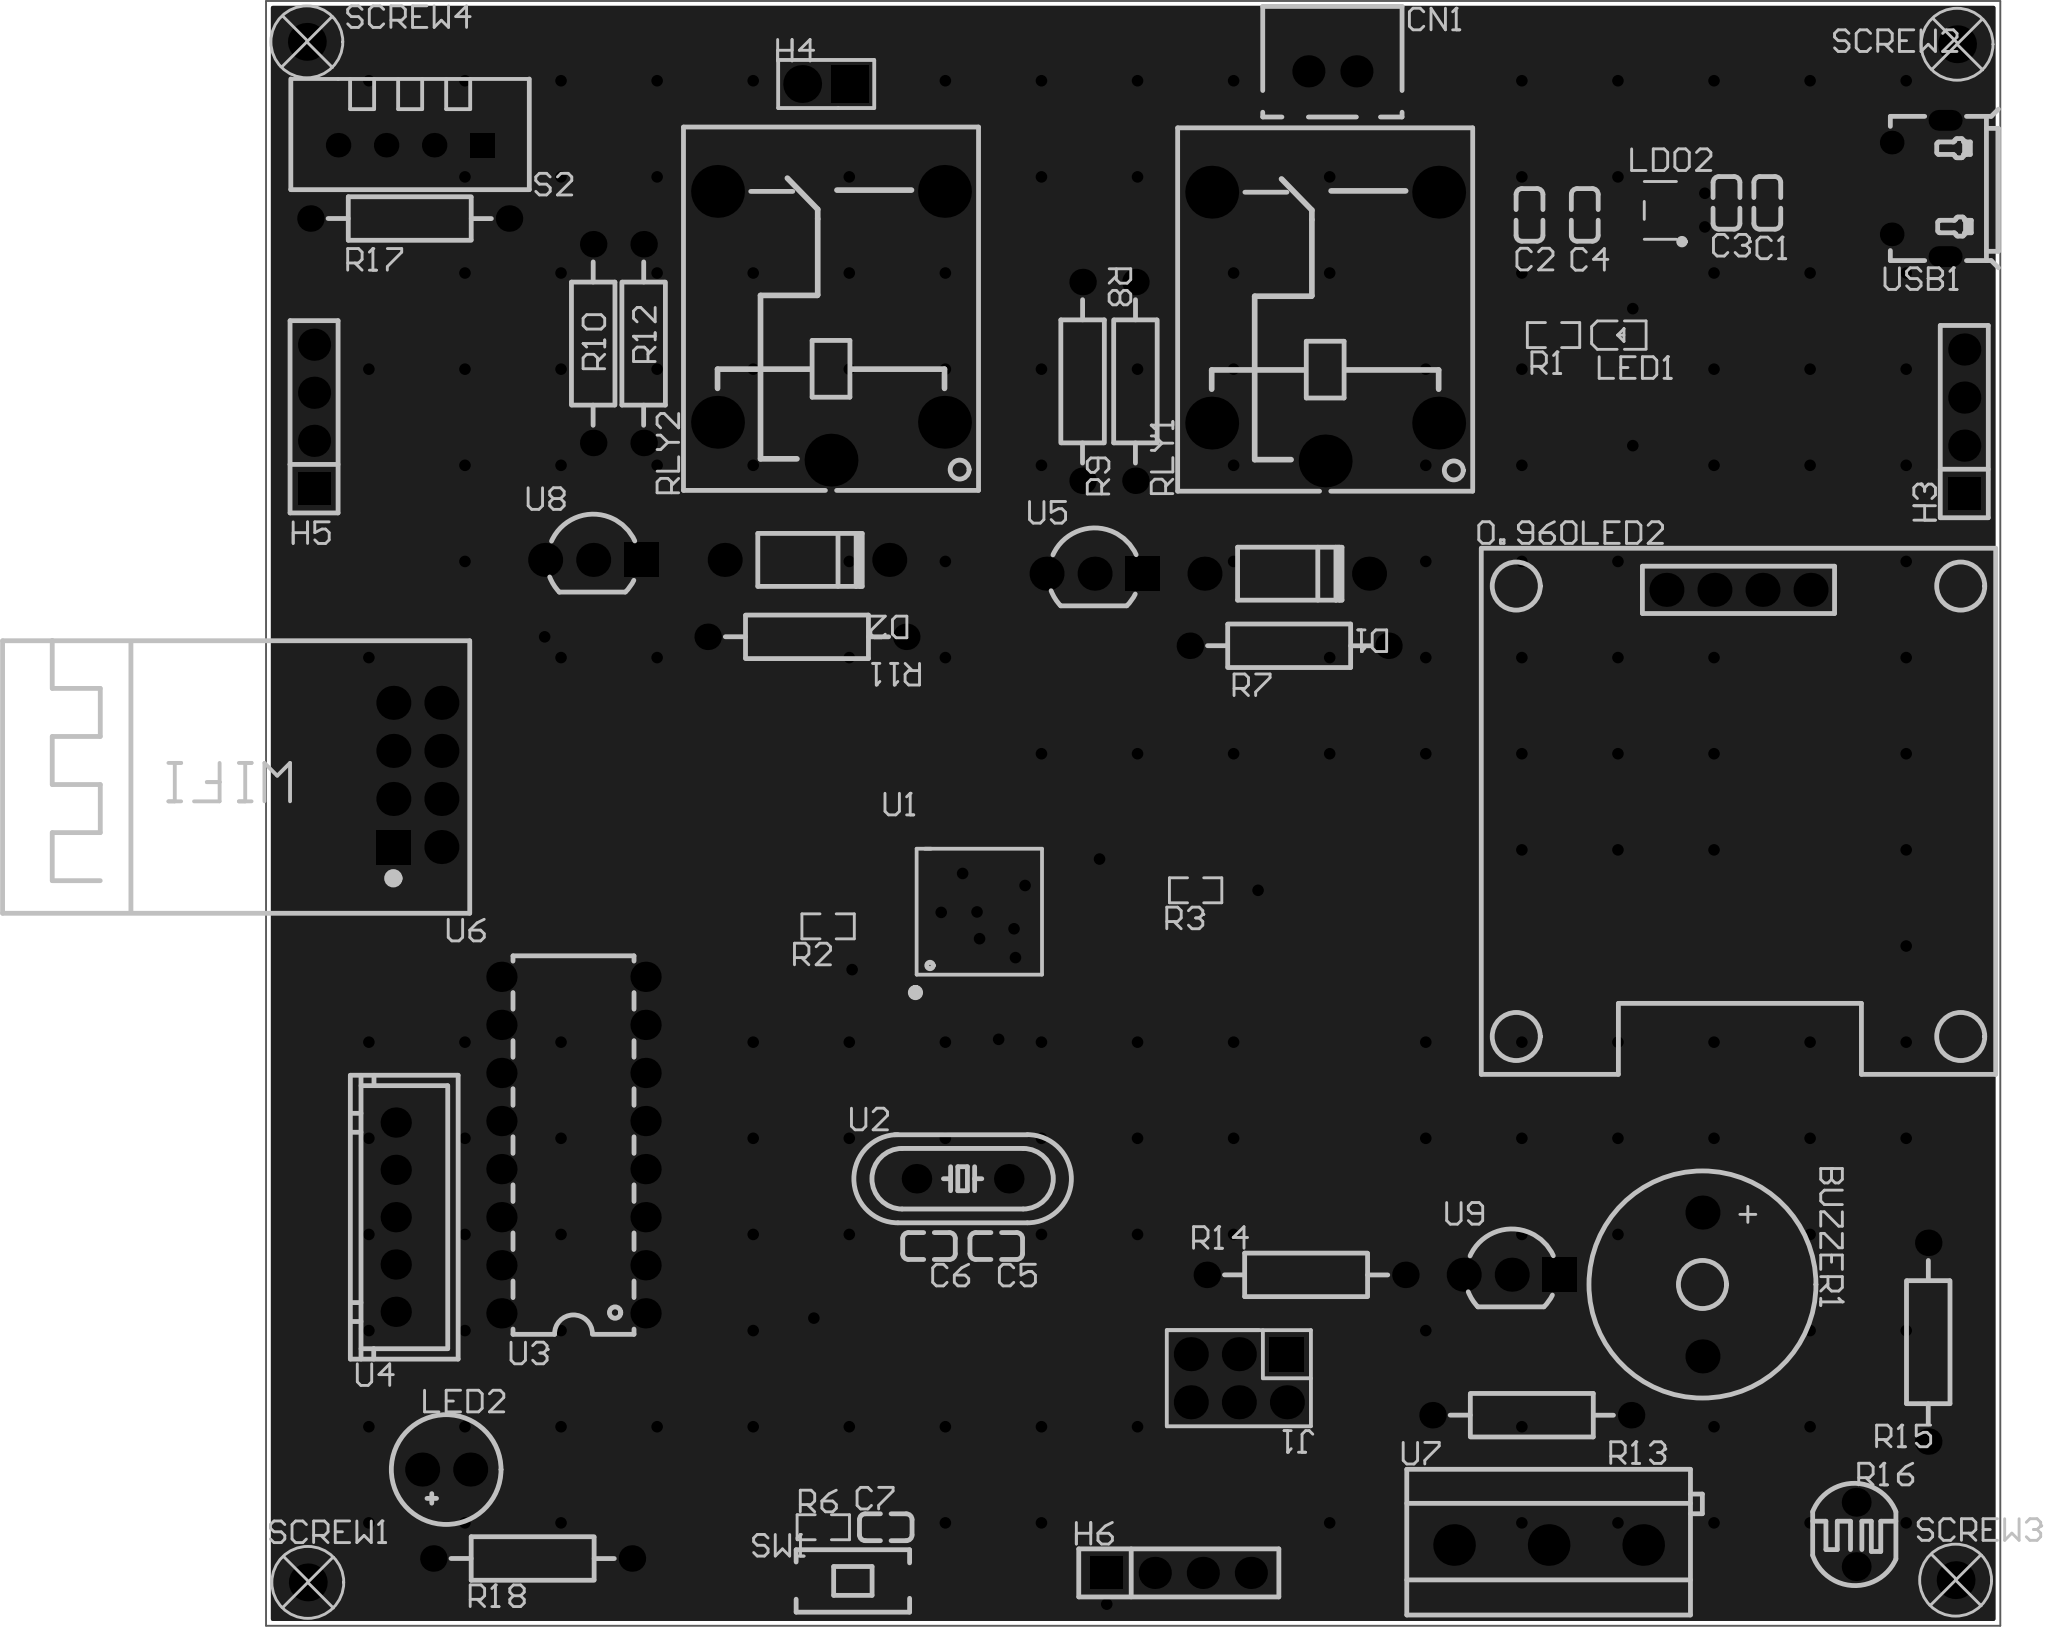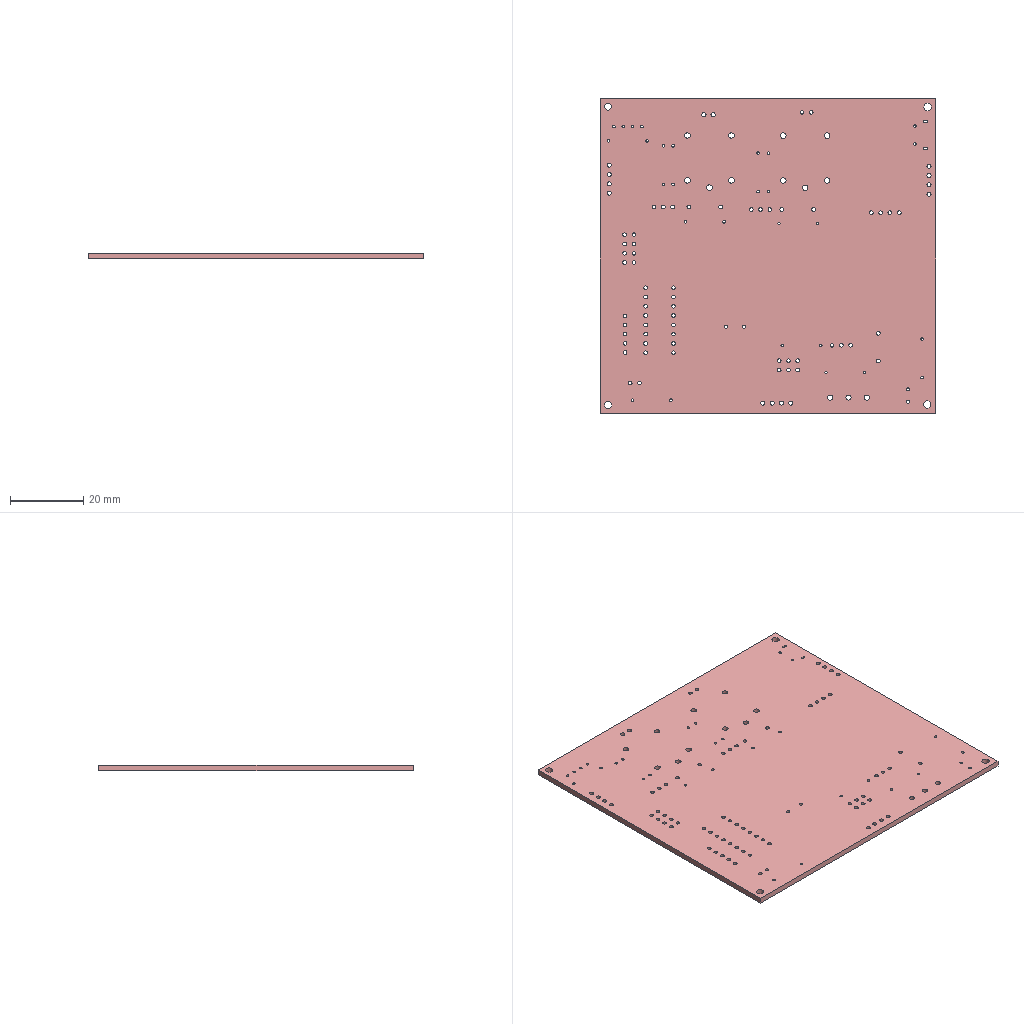Circuit board layout | Altium Designer | box 91.7 x 85.9 x 1.6 mm
Layer stack:
# Altium Designer layer stack of  (unit mm; dielectric type: 0 none, 1 core, 2 prepreg, 3 surface material)
index,name,kind,layer,copper_thickness_mm,dielectric_type,dielectric_thickness_mm,dielectric_material,dielectric_constant
0,Top Paste Mask Layer,other,,,,,,
1,Top Silkscreen Layer,other,,,,,,
2,Top Solder Mask Layer,dielectric,,,3,0.01,,3.3
3,Top Layer,copper,Top Layer,0.035,,,,
4,Dielectric1,dielectric,,,3,1.51,FR4,4.5
5,Bottom Layer,copper,Bottom Layer,0.035,,,,
6,Bottom Solder Mask Layer,dielectric,,,3,0.01,,3.3
7,Bottom Silkscreen Layer,other,,,,,,
8,Bottom Paste Mask Layer,other,,,,,,
# drill layer pairs: low layer,high layer
drill_pair,Top Layer,Bottom Layer
Part placement:
Designator,Comment,Layer,Footprint,Center-X(mm),Center-Y(mm),Rotation
0.96OLED2,,TopLayer,oled-th_l27.8-w27.2-p2.54_c9900033791,168.167,153.416,0
BUZZER1,2.3kHz,TopLayer,BUZ-TH_BD12.0-P7.60-D0.6-FD,166.262,116.713,270
C1,0.1UF,TopLayer,C0603,169.691,173.863,90
C2,0.1UF,TopLayer,C0603,157.118,173.228,270
C3,1uF,TopLayer,C0603,167.532,173.863,90
C4,1uF,TopLayer,C0603,160.039,173.228,270
C5,18pF,TopLayer,C0603,128.924,118.745,180
C6,18pF,TopLayer,C0603,125.368,118.745,180
C7,0.1UF,TopLayer,C0603,123.082,103.886,0
CN1,风扇,TopLayer,CONN-TH_B2B-XH-A-LF-SN,146.697,180.814,0
D1,1N4007,TopLayer,DO-41_BD2.4-L4.7-P8.70-D0.8-RD,144.284,154.271,180
D2,1N4007,TopLayer,DO-41_BD2.4-L4.7-P8.70-D0.8-RD,118.917,154.998,180
H3,JW01,TopLayer,HDR-TH_4P-P2.54-V-M,180.105,162.306,90
H4,水泵,TopLayer,HDR-TH_2P-P2.54-V-M,119.933,180.144,180
H5,串口,TopLayer,HDR-TH_4P-P2.54-V-M,92.856,162.56,90
H6,YL-69,TopLayer,HDR-TH_4P-P2.54-V-F,138.576,101.473,0
J1,2.54-2*3P针,TopLayer,HDR-TH_6P-P2.54-V-M-R2-C3-S2.54-1,141.751,111.76,180
LDO2,ME6211C33M5G-N,TopLayer,SOT-23-5_L3.0-W1.7-P0.95-LS2.8-BL,164.036,173.466,90
LED1,,TopLayer,LED_0603,161.893,166.87,0
LED2,,TopLayer,LED-TH_BD5.9-P2.54-RD,99.841,106.934,180
R1,1kΩ,TopLayer,R0603,158.388,166.878,180
R2,10kΩ,TopLayer,R0603,120.034,135.636,180
R3,10kΩ,TopLayer,R0603,139.465,137.541,180
R6,10kΩ,TopLayer,R0603,119.78,103.886,180
R7,20Ω,TopLayer,RES-TH_BD2.3-L6.5-P10.50-D0.5,144.411,150.461,180
R8,2kΩ,TopLayer,RES-TH_BD2.3-L6.5-P10.50-D0.5,133.489,164.431,270
R9,20kΩ,TopLayer,RES-TH_BD2.3-L6.5-P10.50-D0.5,136.283,164.431,90
R10,2kΩ,TopLayer,RES-TH_BD2.3-L6.5-P10.50-D0.5,107.614,166.428,270
R11,20Ω,TopLayer,RES-TH_BD2.3-L6.5-P10.50-D0.5,118.917,150.934,180
R12,20kΩ,TopLayer,RES-TH_BD2.3-L6.5-P10.50-D0.5,110.281,166.428,90
R13,4.7kΩ,TopLayer,RES-TH_BD2.3-L6.5-P10.50-D0.5,157.24,109.806,180
R14,4.7kΩ,TopLayer,RES-TH_BD2.3-L6.5-P10.50-D0.5,145.307,117.221,0
R15,10kΩ,TopLayer,RES-TH_BD2.3-L6.5-P10.50-D0.5,178.2,113.665,90
R16,GL5528(10-20),TopLayer,RES-TH_L5.1-W4.3-P3.40-D0.5,174.39,103.505,0
R17,4.7kΩ,TopLayer,RES-TH_BD2.3-L6.5-P10.50-D0.5,97.915,173.037,0
R18,150Ω,TopLayer,RES-TH_BD2.3-L6.5-P10.50-D0.5,104.413,102.235,0
RLY1,SRD-05VDC-SL-C,TopLayer,RELAY-TH_SRD-XXVDC-XL-C,146.315,167.328,90
RLY2,SRD-05VDC-SL-C,TopLayer,RELAY-TH_SRD-XXVDC-XL-C,120.188,167.37,90
S2,DHT11,TopLayer,SENSOR-TH_DHT11-1,97.936,176.911,180
SW1,KEY-RESET,TopLayer,SW-SMD_L6.0-W3.3-LS8.0,121.481,101.066,0
U1,STM32F103C8T6,TopLayer,LQFP-48_L7.0-W7.0-P0.50-LS9.0-BL,128.042,136.398,0
U2,8M晶振,TopLayer,HC-49S_L11.5-W4.7-P4.88,127.146,122.301,0
U3,ULN2003A,TopLayer,DIP-16_L20.0-W6.4-P2.54-LS7.6-BL,106.572,124.079,90
U4,步进电机,TopLayer,CONN-TH_5P-P2.50_ZHOURI_XH-5PA,97.174,120.269,90
U5,8050,TopLayer,TO-92-3_L4.8-W3.7-P2.54-R,134.124,154.271,0
U6,2.4GHz,TopLayer,WIFIM-TH_8P-L24.7-W14.4-P2.54,98.317,143.637,180
U7,DS18B20,TopLayer,CONN-TH_3P-P5.00_KF301-5.0-3P,158.129,102.948,0
U8,8050,TopLayer,TO-92-3_L4.8-W3.7-P2.54-R,107.614,154.998,0
U9,8050,TopLayer,TO-92-3_L4.8-W3.7-P2.54-R,156.179,117.23,0
USB1,MICRO-USB-1,TopLayer,MICRO-USB-SMD_C9900008946,177.692,174.625,90
SCREW1,,TopLayer,M2螺丝,92.525,100.971,0
SCREW2,,TopLayer,M2螺丝,179.724,182.245,0
SCREW3,,TopLayer,M2螺丝,179.647,101.091,0
SCREW4,,TopLayer,M2螺丝,92.475,182.372,0
Pad and via stacks:
# Altium Designer via and pad stacks of  (unit mm). Each distinct definition once, with the count of objects using it.
# via: kind,start_layer,end_layer,hole_mm,diameter_mm,mode(0 simple;1 top-mid-bottom;2 full stack),diameter_per_layer,count,example_net
# pad: kind,layer,hole_mm,hole_type(0 round;1 square;2 slot),plating,top_size,top_shape(1 round;2 rect;3 octagon;9 rounded rect),mid_size,bottom_size,mode,footprint,size_per_layer,count,example
pad,Multi-Layer,1.05,0,plated,1.8x1.8,1,1.8x1.8,1.8x1.8,0,oled-th_l27.8-w27.2-p2.54_c9900033791,,4,0.96OLED2.1
pad,Multi-Layer,1,0,plated,1.8x1.8,1,1.8x1.8,1.8x1.8,0,BUZ-TH_BD12.0-P7.60-D0.6-FD,,2,BUZZER1.2
pad,Multi-Layer,1,0,plated,1.7x1.7,1,1.7x1.7,1.7x1.7,0,CONN-TH_B2B-XH-A-LF-SN,,2,CN1.1
pad,Multi-Layer,1.05,0,plated,1.8x1.8,1,1.8x1.8,1.8x1.8,0,DO-41_BD2.4-L4.7-P8.70-D0.8-RD,,4,D1.2
pad,Multi-Layer,1.1,0,plated,1.7x1.7,2,1.7x1.7,1.7x1.7,0,HDR-TH_4P-P2.54-V-M,,2,H3.1
pad,Multi-Layer,1.1,0,plated,1.7x1.7,1,1.7x1.7,1.7x1.7,0,HDR-TH_4P-P2.54-V-M,,6,H3.2
pad,Multi-Layer,1.2,0,plated,2x2,2,2x2,2x2,0,HDR-TH_2P-P2.54-V-M,,1,H4.1
pad,Multi-Layer,1.2,0,plated,2x2,1,2x2,2x2,0,HDR-TH_2P-P2.54-V-M,,1,H4.2
pad,Multi-Layer,1.1,0,plated,1.7x1.7,2,1.7x1.7,1.7x1.7,0,HDR-TH_4P-P2.54-V-F,,1,H6.1
pad,Multi-Layer,1.1,0,plated,1.7x1.7,1,1.7x1.7,1.7x1.7,0,HDR-TH_4P-P2.54-V-F,,3,H6.2
pad,Multi-Layer,1.05,0,plated,1.8x1.8,1,1.8x1.8,1.8x1.8,0,HDR-TH_6P-P2.54-V-M-R2-C3-S2.54-1,,5,J1.6
pad,Multi-Layer,1.05,0,plated,1.8x1.8,2,1.8x1.8,1.8x1.8,0,HDR-TH_6P-P2.54-V-M-R2-C3-S2.54-1,,1,J1.1
pad,Multi-Layer,1,0,plated,1.8x1.8,1,1.8x1.8,1.8x1.8,0,LED-TH_BD5.9-P2.54-RD,,2,LED2.1
pad,Multi-Layer,0.7,0,plated,1.4x1.4,1,1.4x1.4,1.4x1.4,0,RES-TH_BD2.3-L6.5-P10.50-D0.5,,22,R7.1
pad,Multi-Layer,0.762,0,plated,1.524x1.524,1,1.524x1.524,1.524x1.524,0,RES-TH_L5.1-W4.3-P3.40-D0.5,,2,R16.2
pad,Multi-Layer,1.524,0,plated,2.794x2.794,1,2.794x2.794,2.794x2.794,0,RELAY-TH_SRD-XXVDC-XL-C,,10,RLY1.2
pad,Multi-Layer,0.7112,0,plated,1.295x1.295,1,1.295x1.295,1.295x1.295,0,SENSOR-TH_DHT11-1,,3,S2.4
pad,Multi-Layer,0.7112,0,plated,1.295x1.295,2,1.295x1.295,1.295x1.295,0,SENSOR-TH_DHT11-1,,1,S2.1
pad,Multi-Layer,0.9,0,plated,1.56x1.56,1,1.56x1.56,1.56x1.56,0,HC-49S_L11.5-W4.7-P4.88,,2,U2.2
pad,Multi-Layer,1,0,plated,1.6x1.6,1,1.6x1.6,1.6x1.6,0,DIP-16_L20.0-W6.4-P2.54-LS7.6-BL,,16,U3.1
pad,Multi-Layer,1,0,plated,1.6x1.6,1,1.6x1.6,1.6x1.6,0,CONN-TH_5P-P2.50_ZHOURI_XH-5PA,,5,U4.1
pad,Multi-Layer,1,0,plated,1.8x1.8,2,1.8x1.8,1.8x1.8,0,TO-92-3_L4.8-W3.7-P2.54-R,,3,U5.1
pad,Multi-Layer,1,0,plated,1.8x1.8,1,1.8x1.8,1.8x1.8,0,TO-92-3_L4.8-W3.7-P2.54-R,,6,U5.2
pad,Multi-Layer,1,0,plated,1.8x1.8,1,1.8x1.8,1.8x1.8,0,WIFIM-TH_8P-L24.7-W14.4-P2.54,,7,U6.8
pad,Multi-Layer,1,0,plated,1.8x1.8,2,1.8x1.8,1.8x1.8,0,WIFIM-TH_8P-L24.7-W14.4-P2.54,,1,U6.1
pad,Multi-Layer,1.4,0,plated,2.2x2.2,1,2.2x2.2,2.2x2.2,0,CONN-TH_3P-P5.00_KF301-5.0-3P,,3,U7.1
pad,Multi-Layer,0.7,0,plated,1.25x1.25,1,1.25x1.25,1.25x1.25,0,MICRO-USB-SMD_C9900008946,,2,USB1.6
pad,Multi-Layer,0.6,2,plated,1.1x1.8,1,1.1x1.8,1.1x1.8,0,MICRO-USB-SMD_C9900008946,,2,USB1.6
pad,Multi-Layer,2,0,plated,2x2,1,2x2,2x2,0,M2\u00C2\u00DD\u00CB\u00BF,,4,SCREW1.1
pad,Top Layer,0,0,plated,0.8x0.9,2,0.8x0.9,0.8x0.9,0,C0603,,14,C1.2
pad,Top Layer,0,0,plated,0.49x1.157,2,0.49x1.157,0.49x1.157,0,SOT-23-5_L3.0-W1.7-P0.95-LS2.8-BL,,3,LDO2.1
pad,Top Layer,0,0,plated,0.49x1.175,2,0.49x1.175,0.49x1.175,0,SOT-23-5_L3.0-W1.7-P0.95-LS2.8-BL,,2,LDO2.4
pad,Top Layer,0,0,plated,0.8001x0.8001,2,0.8001x0.8001,0.8001x0.8001,0,LED_0603,,2,LED1.1
pad,Top Layer,0,0,plated,0.8065x0.864,2,0.8065x0.864,0.8065x0.864,0,R0603,,8,R1.2
pad,Top Layer,0,0,plated,1.9x1.5,2,1.9x1.5,1.9x1.5,0,SW-SMD_L6.0-W3.3-LS8.0,,2,SW1.1
pad,Top Layer,0,0,plated,0.27x1.5,1,0.27x1.5,0.27x1.5,0,LQFP-48_L7.0-W7.0-P0.50-LS9.0-BL,,24,U1.1
pad,Top Layer,0,0,plated,1.5x0.27,1,1.5x0.27,1.5x0.27,0,LQFP-48_L7.0-W7.0-P0.50-LS9.0-BL,,24,U1.13
pad,Top Layer,0,0,plated,1.35x0.4,2,1.35x0.4,1.35x0.4,0,MICRO-USB-SMD_C9900008946,,5,USB1.1
via,Top Layer,Bottom Layer,0.3048,0.61,0,,183,PA2
Copper pours:
name,layer,net,type(0 solid;1 hatched;2 none)
Bottom Layer-GND,Bottom Layer,GND,0
Top Layer-GND,Top Layer,GND,0